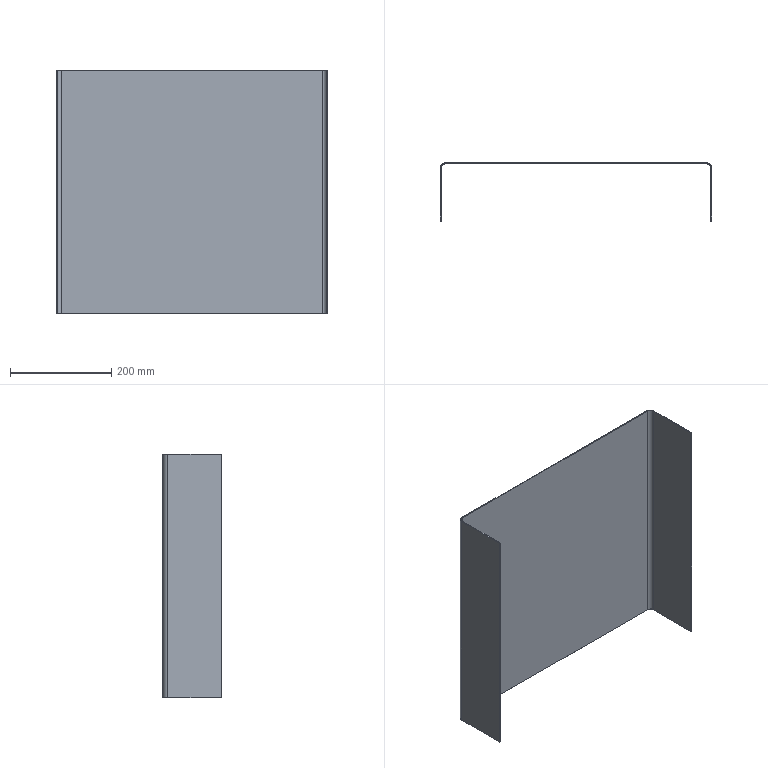Part | SolidWorks | features ExtruThin 1 | 1 solid | 14 faces | box 536 x 115.5 x 480 mm | volume 725063 mm3 | plane 10 | cylinder 4 | commonest cylinder face diameters 16 x2 20 x2
STEP:
#1=CARTESIAN_POINT('',(0.,-10.,0.));
#2=VERTEX_POINT('',#1);
#3=CARTESIAN_POINT('',(0.,-115.5,0.));
#4=VERTEX_POINT('',#3);
#5=CARTESIAN_POINT('',(0.,-10.,0.));
#6=DIRECTION('',(0.,-1.,0.));
#7=VECTOR('',#6,1000.);
#8=LINE('',#5,#7);
#9=EDGE_CURVE('',#2,#4,#8,.T.);
#10=ORIENTED_EDGE('',*,*,#9,.T.);
#11=CARTESIAN_POINT('',(0.,-115.5,480.));
#12=VERTEX_POINT('',#11);
#13=CARTESIAN_POINT('',(0.,-115.5,480.));
#14=DIRECTION('',(0.,0.,-1.));
#15=VECTOR('',#14,1000.);
#16=LINE('',#13,#15);
#17=EDGE_CURVE('',#12,#4,#16,.T.);
#18=ORIENTED_EDGE('',*,*,#17,.F.);
#19=CARTESIAN_POINT('',(0.,-10.,480.));
#20=VERTEX_POINT('',#19);
#21=CARTESIAN_POINT('',(0.,-10.,480.));
#22=DIRECTION('',(0.,-1.,0.));
#23=VECTOR('',#22,1000.);
#24=LINE('',#21,#23);
#25=EDGE_CURVE('',#20,#12,#24,.T.);
#26=ORIENTED_EDGE('',*,*,#25,.F.);
#27=CARTESIAN_POINT('',(0.,-10.,480.));
#28=DIRECTION('',(0.,0.,-1.));
#29=VECTOR('',#28,1000.);
#30=LINE('',#27,#29);
#31=EDGE_CURVE('',#20,#2,#30,.T.);
#32=ORIENTED_EDGE('',*,*,#31,.T.);
#33=EDGE_LOOP('',(#10,#18,#26,#32));
#34=FACE_OUTER_BOUND('',#33,.T.);
#35=CARTESIAN_POINT('',(0.,-10.,480.));
#36=DIRECTION('',(1.,0.,0.));
#37=DIRECTION('',(0.,1.,0.));
#38=AXIS2_PLACEMENT_3D('',#35,#36,#37);
#39=PLANE('',#38);
#40=ADVANCED_FACE('',(#34),#39,.F.);
#41=CARTESIAN_POINT('',(2.,-115.5,0.));
#42=VERTEX_POINT('',#41);
#43=CARTESIAN_POINT('',(2.,-115.5,0.));
#44=DIRECTION('',(-1.,0.,0.));
#45=VECTOR('',#44,1000.);
#46=LINE('',#43,#45);
#47=EDGE_CURVE('',#42,#4,#46,.T.);
#48=ORIENTED_EDGE('',*,*,#47,.F.);
#49=CARTESIAN_POINT('',(2.,-115.5,480.));
#50=VERTEX_POINT('',#49);
#51=CARTESIAN_POINT('',(2.,-115.5,480.));
#52=DIRECTION('',(0.,0.,-1.));
#53=VECTOR('',#52,1000.);
#54=LINE('',#51,#53);
#55=EDGE_CURVE('',#50,#42,#54,.T.);
#56=ORIENTED_EDGE('',*,*,#55,.F.);
#57=CARTESIAN_POINT('',(2.,-115.5,480.));
#58=DIRECTION('',(-1.,0.,0.));
#59=VECTOR('',#58,1000.);
#60=LINE('',#57,#59);
#61=EDGE_CURVE('',#50,#12,#60,.T.);
#62=ORIENTED_EDGE('',*,*,#61,.T.);
#63=ORIENTED_EDGE('',*,*,#17,.T.);
#64=EDGE_LOOP('',(#48,#56,#62,#63));
#65=FACE_OUTER_BOUND('',#64,.T.);
#66=CARTESIAN_POINT('',(2.,-115.5,480.));
#67=DIRECTION('',(0.,-1.,0.));
#68=DIRECTION('',(1.,0.,0.));
#69=AXIS2_PLACEMENT_3D('',#66,#67,#68);
#70=PLANE('',#69);
#71=ADVANCED_FACE('',(#65),#70,.T.);
#72=CARTESIAN_POINT('',(2.,-10.,0.));
#73=VERTEX_POINT('',#72);
#74=CARTESIAN_POINT('',(2.,-10.,0.));
#75=DIRECTION('',(0.,-1.,0.));
#76=VECTOR('',#75,1000.);
#77=LINE('',#74,#76);
#78=EDGE_CURVE('',#73,#42,#77,.T.);
#79=ORIENTED_EDGE('',*,*,#78,.F.);
#80=CARTESIAN_POINT('',(2.,-10.,480.));
#81=VERTEX_POINT('',#80);
#82=CARTESIAN_POINT('',(2.,-10.,480.));
#83=DIRECTION('',(0.,0.,-1.));
#84=VECTOR('',#83,1000.);
#85=LINE('',#82,#84);
#86=EDGE_CURVE('',#81,#73,#85,.T.);
#87=ORIENTED_EDGE('',*,*,#86,.F.);
#88=CARTESIAN_POINT('',(2.,-10.,480.));
#89=DIRECTION('',(0.,-1.,0.));
#90=VECTOR('',#89,1000.);
#91=LINE('',#88,#90);
#92=EDGE_CURVE('',#81,#50,#91,.T.);
#93=ORIENTED_EDGE('',*,*,#92,.T.);
#94=ORIENTED_EDGE('',*,*,#55,.T.);
#95=EDGE_LOOP('',(#79,#87,#93,#94));
#96=FACE_OUTER_BOUND('',#95,.T.);
#97=CARTESIAN_POINT('',(2.,-10.,480.));
#98=DIRECTION('',(1.,0.,0.));
#99=DIRECTION('',(0.,1.,0.));
#100=AXIS2_PLACEMENT_3D('',#97,#98,#99);
#101=PLANE('',#100);
#102=ADVANCED_FACE('',(#96),#101,.T.);
#103=CARTESIAN_POINT('',(10.,-2.,0.));
#104=VERTEX_POINT('',#103);
#105=CARTESIAN_POINT('',(10.,-10.,0.));
#106=DIRECTION('',(0.,0.,1.));
#107=DIRECTION('',(1.,0.,0.));
#108=AXIS2_PLACEMENT_3D('',#105,#106,#107);
#109=CIRCLE('',#108,8.);
#110=EDGE_CURVE('',#104,#73,#109,.T.);
#111=ORIENTED_EDGE('',*,*,#110,.F.);
#112=CARTESIAN_POINT('',(10.,-2.,480.));
#113=VERTEX_POINT('',#112);
#114=CARTESIAN_POINT('',(10.,-2.,480.));
#115=DIRECTION('',(0.,0.,-1.));
#116=VECTOR('',#115,1000.);
#117=LINE('',#114,#116);
#118=EDGE_CURVE('',#113,#104,#117,.T.);
#119=ORIENTED_EDGE('',*,*,#118,.F.);
#120=CARTESIAN_POINT('',(10.,-10.,480.));
#121=DIRECTION('',(0.,0.,1.));
#122=DIRECTION('',(1.,0.,0.));
#123=AXIS2_PLACEMENT_3D('',#120,#121,#122);
#124=CIRCLE('',#123,8.);
#125=EDGE_CURVE('',#113,#81,#124,.T.);
#126=ORIENTED_EDGE('',*,*,#125,.T.);
#127=ORIENTED_EDGE('',*,*,#86,.T.);
#128=EDGE_LOOP('',(#111,#119,#126,#127));
#129=FACE_OUTER_BOUND('',#128,.T.);
#130=CARTESIAN_POINT('',(10.,-10.,480.));
#131=DIRECTION('',(0.,0.,-1.));
#132=DIRECTION('',(-1.,0.,0.));
#133=AXIS2_PLACEMENT_3D('',#130,#131,#132);
#134=CYLINDRICAL_SURFACE('',#133,8.);
#135=ADVANCED_FACE('',(#129),#134,.F.);
#136=CARTESIAN_POINT('',(526.,-2.,0.));
#137=VERTEX_POINT('',#136);
#138=CARTESIAN_POINT('',(10.,-2.,0.));
#139=DIRECTION('',(-1.,0.,0.));
#140=VECTOR('',#139,1000.);
#141=LINE('',#138,#140);
#142=EDGE_CURVE('',#137,#104,#141,.T.);
#143=ORIENTED_EDGE('',*,*,#142,.F.);
#144=CARTESIAN_POINT('',(526.,-2.,480.));
#145=VERTEX_POINT('',#144);
#146=CARTESIAN_POINT('',(526.,-2.,480.));
#147=DIRECTION('',(0.,0.,-1.));
#148=VECTOR('',#147,1000.);
#149=LINE('',#146,#148);
#150=EDGE_CURVE('',#145,#137,#149,.T.);
#151=ORIENTED_EDGE('',*,*,#150,.F.);
#152=CARTESIAN_POINT('',(10.,-2.,480.));
#153=DIRECTION('',(-1.,0.,0.));
#154=VECTOR('',#153,1000.);
#155=LINE('',#152,#154);
#156=EDGE_CURVE('',#145,#113,#155,.T.);
#157=ORIENTED_EDGE('',*,*,#156,.T.);
#158=ORIENTED_EDGE('',*,*,#118,.T.);
#159=EDGE_LOOP('',(#143,#151,#157,#158));
#160=FACE_OUTER_BOUND('',#159,.T.);
#161=CARTESIAN_POINT('',(10.,-2.,480.));
#162=DIRECTION('',(0.,-1.,0.));
#163=DIRECTION('',(0.,0.,-1.));
#164=AXIS2_PLACEMENT_3D('',#161,#162,#163);
#165=PLANE('',#164);
#166=ADVANCED_FACE('',(#160),#165,.T.);
#167=CARTESIAN_POINT('',(534.,-10.,0.));
#168=VERTEX_POINT('',#167);
#169=CARTESIAN_POINT('',(526.,-10.,0.));
#170=DIRECTION('',(0.,0.,1.));
#171=DIRECTION('',(1.,0.,0.));
#172=AXIS2_PLACEMENT_3D('',#169,#170,#171);
#173=CIRCLE('',#172,8.);
#174=EDGE_CURVE('',#168,#137,#173,.T.);
#175=ORIENTED_EDGE('',*,*,#174,.F.);
#176=CARTESIAN_POINT('',(534.,-10.,480.));
#177=VERTEX_POINT('',#176);
#178=CARTESIAN_POINT('',(534.,-10.,480.));
#179=DIRECTION('',(0.,0.,-1.));
#180=VECTOR('',#179,1000.);
#181=LINE('',#178,#180);
#182=EDGE_CURVE('',#177,#168,#181,.T.);
#183=ORIENTED_EDGE('',*,*,#182,.F.);
#184=CARTESIAN_POINT('',(526.,-10.,480.));
#185=DIRECTION('',(0.,0.,1.));
#186=DIRECTION('',(1.,0.,0.));
#187=AXIS2_PLACEMENT_3D('',#184,#185,#186);
#188=CIRCLE('',#187,8.);
#189=EDGE_CURVE('',#177,#145,#188,.T.);
#190=ORIENTED_EDGE('',*,*,#189,.T.);
#191=ORIENTED_EDGE('',*,*,#150,.T.);
#192=EDGE_LOOP('',(#175,#183,#190,#191));
#193=FACE_OUTER_BOUND('',#192,.T.);
#194=CARTESIAN_POINT('',(526.,-10.,480.));
#195=DIRECTION('',(0.,0.,-1.));
#196=DIRECTION('',(-1.,0.,0.));
#197=AXIS2_PLACEMENT_3D('',#194,#195,#196);
#198=CYLINDRICAL_SURFACE('',#197,8.);
#199=ADVANCED_FACE('',(#193),#198,.F.);
#200=CARTESIAN_POINT('',(534.,-115.5,0.));
#201=VERTEX_POINT('',#200);
#202=CARTESIAN_POINT('',(534.,-10.,0.));
#203=DIRECTION('',(0.,1.,0.));
#204=VECTOR('',#203,1000.);
#205=LINE('',#202,#204);
#206=EDGE_CURVE('',#201,#168,#205,.T.);
#207=ORIENTED_EDGE('',*,*,#206,.F.);
#208=CARTESIAN_POINT('',(534.,-115.5,480.));
#209=VERTEX_POINT('',#208);
#210=CARTESIAN_POINT('',(534.,-115.5,480.));
#211=DIRECTION('',(0.,0.,-1.));
#212=VECTOR('',#211,1000.);
#213=LINE('',#210,#212);
#214=EDGE_CURVE('',#209,#201,#213,.T.);
#215=ORIENTED_EDGE('',*,*,#214,.F.);
#216=CARTESIAN_POINT('',(534.,-10.,480.));
#217=DIRECTION('',(0.,1.,0.));
#218=VECTOR('',#217,1000.);
#219=LINE('',#216,#218);
#220=EDGE_CURVE('',#209,#177,#219,.T.);
#221=ORIENTED_EDGE('',*,*,#220,.T.);
#222=ORIENTED_EDGE('',*,*,#182,.T.);
#223=EDGE_LOOP('',(#207,#215,#221,#222));
#224=FACE_OUTER_BOUND('',#223,.T.);
#225=CARTESIAN_POINT('',(534.,-10.,480.));
#226=DIRECTION('',(-1.,0.,0.));
#227=DIRECTION('',(0.,0.,1.));
#228=AXIS2_PLACEMENT_3D('',#225,#226,#227);
#229=PLANE('',#228);
#230=ADVANCED_FACE('',(#224),#229,.T.);
#231=CARTESIAN_POINT('',(536.,-115.5,0.));
#232=VERTEX_POINT('',#231);
#233=CARTESIAN_POINT('',(536.,-115.5,0.));
#234=DIRECTION('',(-1.,0.,0.));
#235=VECTOR('',#234,1000.);
#236=LINE('',#233,#235);
#237=EDGE_CURVE('',#232,#201,#236,.T.);
#238=ORIENTED_EDGE('',*,*,#237,.F.);
#239=CARTESIAN_POINT('',(536.,-115.5,480.));
#240=VERTEX_POINT('',#239);
#241=CARTESIAN_POINT('',(536.,-115.5,480.));
#242=DIRECTION('',(0.,0.,-1.));
#243=VECTOR('',#242,1000.);
#244=LINE('',#241,#243);
#245=EDGE_CURVE('',#240,#232,#244,.T.);
#246=ORIENTED_EDGE('',*,*,#245,.F.);
#247=CARTESIAN_POINT('',(536.,-115.5,480.));
#248=DIRECTION('',(-1.,0.,0.));
#249=VECTOR('',#248,1000.);
#250=LINE('',#247,#249);
#251=EDGE_CURVE('',#240,#209,#250,.T.);
#252=ORIENTED_EDGE('',*,*,#251,.T.);
#253=ORIENTED_EDGE('',*,*,#214,.T.);
#254=EDGE_LOOP('',(#238,#246,#252,#253));
#255=FACE_OUTER_BOUND('',#254,.T.);
#256=CARTESIAN_POINT('',(536.,-115.5,480.));
#257=DIRECTION('',(0.,-1.,0.));
#258=DIRECTION('',(0.,0.,-1.));
#259=AXIS2_PLACEMENT_3D('',#256,#257,#258);
#260=PLANE('',#259);
#261=ADVANCED_FACE('',(#255),#260,.T.);
#262=CARTESIAN_POINT('',(536.,-10.,0.));
#263=VERTEX_POINT('',#262);
#264=CARTESIAN_POINT('',(536.,-10.,0.));
#265=DIRECTION('',(0.,1.,0.));
#266=VECTOR('',#265,1000.);
#267=LINE('',#264,#266);
#268=EDGE_CURVE('',#232,#263,#267,.T.);
#269=ORIENTED_EDGE('',*,*,#268,.T.);
#270=CARTESIAN_POINT('',(536.,-10.,480.));
#271=VERTEX_POINT('',#270);
#272=CARTESIAN_POINT('',(536.,-10.,480.));
#273=DIRECTION('',(0.,0.,-1.));
#274=VECTOR('',#273,1000.);
#275=LINE('',#272,#274);
#276=EDGE_CURVE('',#271,#263,#275,.T.);
#277=ORIENTED_EDGE('',*,*,#276,.F.);
#278=CARTESIAN_POINT('',(536.,-10.,480.));
#279=DIRECTION('',(0.,1.,0.));
#280=VECTOR('',#279,1000.);
#281=LINE('',#278,#280);
#282=EDGE_CURVE('',#240,#271,#281,.T.);
#283=ORIENTED_EDGE('',*,*,#282,.F.);
#284=ORIENTED_EDGE('',*,*,#245,.T.);
#285=EDGE_LOOP('',(#269,#277,#283,#284));
#286=FACE_OUTER_BOUND('',#285,.T.);
#287=CARTESIAN_POINT('',(536.,-10.,480.));
#288=DIRECTION('',(-1.,0.,0.));
#289=DIRECTION('',(0.,0.,1.));
#290=AXIS2_PLACEMENT_3D('',#287,#288,#289);
#291=PLANE('',#290);
#292=ADVANCED_FACE('',(#286),#291,.F.);
#293=CARTESIAN_POINT('',(526.,0.,0.));
#294=VERTEX_POINT('',#293);
#295=CARTESIAN_POINT('',(526.,-10.,0.));
#296=DIRECTION('',(0.,0.,1.));
#297=DIRECTION('',(1.,0.,0.));
#298=AXIS2_PLACEMENT_3D('',#295,#296,#297);
#299=CIRCLE('',#298,10.);
#300=EDGE_CURVE('',#263,#294,#299,.T.);
#301=ORIENTED_EDGE('',*,*,#300,.T.);
#302=CARTESIAN_POINT('',(526.,0.,480.));
#303=VERTEX_POINT('',#302);
#304=CARTESIAN_POINT('',(526.,0.,480.));
#305=DIRECTION('',(0.,0.,-1.));
#306=VECTOR('',#305,1000.);
#307=LINE('',#304,#306);
#308=EDGE_CURVE('',#303,#294,#307,.T.);
#309=ORIENTED_EDGE('',*,*,#308,.F.);
#310=CARTESIAN_POINT('',(526.,-10.,480.));
#311=DIRECTION('',(0.,0.,1.));
#312=DIRECTION('',(1.,0.,0.));
#313=AXIS2_PLACEMENT_3D('',#310,#311,#312);
#314=CIRCLE('',#313,10.);
#315=EDGE_CURVE('',#271,#303,#314,.T.);
#316=ORIENTED_EDGE('',*,*,#315,.F.);
#317=ORIENTED_EDGE('',*,*,#276,.T.);
#318=EDGE_LOOP('',(#301,#309,#316,#317));
#319=FACE_OUTER_BOUND('',#318,.T.);
#320=CARTESIAN_POINT('',(526.,-10.,480.));
#321=DIRECTION('',(0.,0.,-1.));
#322=DIRECTION('',(-1.,0.,0.));
#323=AXIS2_PLACEMENT_3D('',#320,#321,#322);
#324=CYLINDRICAL_SURFACE('',#323,10.);
#325=ADVANCED_FACE('',(#319),#324,.T.);
#326=CARTESIAN_POINT('',(10.,0.,0.));
#327=VERTEX_POINT('',#326);
#328=CARTESIAN_POINT('',(10.,0.,0.));
#329=DIRECTION('',(-1.,0.,0.));
#330=VECTOR('',#329,1000.);
#331=LINE('',#328,#330);
#332=EDGE_CURVE('',#294,#327,#331,.T.);
#333=ORIENTED_EDGE('',*,*,#332,.T.);
#334=CARTESIAN_POINT('',(10.,0.,480.));
#335=VERTEX_POINT('',#334);
#336=CARTESIAN_POINT('',(10.,0.,480.));
#337=DIRECTION('',(0.,0.,-1.));
#338=VECTOR('',#337,1000.);
#339=LINE('',#336,#338);
#340=EDGE_CURVE('',#335,#327,#339,.T.);
#341=ORIENTED_EDGE('',*,*,#340,.F.);
#342=CARTESIAN_POINT('',(10.,0.,480.));
#343=DIRECTION('',(-1.,0.,0.));
#344=VECTOR('',#343,1000.);
#345=LINE('',#342,#344);
#346=EDGE_CURVE('',#303,#335,#345,.T.);
#347=ORIENTED_EDGE('',*,*,#346,.F.);
#348=ORIENTED_EDGE('',*,*,#308,.T.);
#349=EDGE_LOOP('',(#333,#341,#347,#348));
#350=FACE_OUTER_BOUND('',#349,.T.);
#351=CARTESIAN_POINT('',(10.,0.,480.));
#352=DIRECTION('',(0.,-1.,0.));
#353=DIRECTION('',(0.,0.,-1.));
#354=AXIS2_PLACEMENT_3D('',#351,#352,#353);
#355=PLANE('',#354);
#356=ADVANCED_FACE('',(#350),#355,.F.);
#357=CARTESIAN_POINT('',(10.,-10.,0.));
#358=DIRECTION('',(0.,0.,1.));
#359=DIRECTION('',(1.,0.,0.));
#360=AXIS2_PLACEMENT_3D('',#357,#358,#359);
#361=CIRCLE('',#360,10.);
#362=EDGE_CURVE('',#327,#2,#361,.T.);
#363=ORIENTED_EDGE('',*,*,#362,.T.);
#364=ORIENTED_EDGE('',*,*,#31,.F.);
#365=CARTESIAN_POINT('',(10.,-10.,480.));
#366=DIRECTION('',(0.,0.,1.));
#367=DIRECTION('',(1.,0.,0.));
#368=AXIS2_PLACEMENT_3D('',#365,#366,#367);
#369=CIRCLE('',#368,10.);
#370=EDGE_CURVE('',#335,#20,#369,.T.);
#371=ORIENTED_EDGE('',*,*,#370,.F.);
#372=ORIENTED_EDGE('',*,*,#340,.T.);
#373=EDGE_LOOP('',(#363,#364,#371,#372));
#374=FACE_OUTER_BOUND('',#373,.T.);
#375=CARTESIAN_POINT('',(10.,-10.,480.));
#376=DIRECTION('',(0.,0.,-1.));
#377=DIRECTION('',(-1.,0.,0.));
#378=AXIS2_PLACEMENT_3D('',#375,#376,#377);
#379=CYLINDRICAL_SURFACE('',#378,10.);
#380=ADVANCED_FACE('',(#374),#379,.T.);
#381=ORIENTED_EDGE('',*,*,#25,.T.);
#382=ORIENTED_EDGE('',*,*,#61,.F.);
#383=ORIENTED_EDGE('',*,*,#92,.F.);
#384=ORIENTED_EDGE('',*,*,#125,.F.);
#385=ORIENTED_EDGE('',*,*,#156,.F.);
#386=ORIENTED_EDGE('',*,*,#189,.F.);
#387=ORIENTED_EDGE('',*,*,#220,.F.);
#388=ORIENTED_EDGE('',*,*,#251,.F.);
#389=ORIENTED_EDGE('',*,*,#282,.T.);
#390=ORIENTED_EDGE('',*,*,#315,.T.);
#391=ORIENTED_EDGE('',*,*,#346,.T.);
#392=ORIENTED_EDGE('',*,*,#370,.T.);
#393=EDGE_LOOP('',(#381,#382,#383,#384,#385,#386,#387,#388,#389,#390,#391,#392));
#394=FACE_OUTER_BOUND('',#393,.T.);
#395=CARTESIAN_POINT('',(10.,-10.,480.));
#396=DIRECTION('',(0.,0.,1.));
#397=DIRECTION('',(1.,0.,0.));
#398=AXIS2_PLACEMENT_3D('',#395,#396,#397);
#399=PLANE('',#398);
#400=ADVANCED_FACE('',(#394),#399,.T.);
#401=ORIENTED_EDGE('',*,*,#9,.F.);
#402=ORIENTED_EDGE('',*,*,#362,.F.);
#403=ORIENTED_EDGE('',*,*,#332,.F.);
#404=ORIENTED_EDGE('',*,*,#300,.F.);
#405=ORIENTED_EDGE('',*,*,#268,.F.);
#406=ORIENTED_EDGE('',*,*,#237,.T.);
#407=ORIENTED_EDGE('',*,*,#206,.T.);
#408=ORIENTED_EDGE('',*,*,#174,.T.);
#409=ORIENTED_EDGE('',*,*,#142,.T.);
#410=ORIENTED_EDGE('',*,*,#110,.T.);
#411=ORIENTED_EDGE('',*,*,#78,.T.);
#412=ORIENTED_EDGE('',*,*,#47,.T.);
#413=EDGE_LOOP('',(#401,#402,#403,#404,#405,#406,#407,#408,#409,#410,#411,#412));
#414=FACE_OUTER_BOUND('',#413,.T.);
#415=CARTESIAN_POINT('',(10.,-10.,0.));
#416=DIRECTION('',(0.,0.,1.));
#417=DIRECTION('',(1.,0.,0.));
#418=AXIS2_PLACEMENT_3D('',#415,#416,#417);
#419=PLANE('',#418);
#420=ADVANCED_FACE('',(#414),#419,.F.);
#421=CLOSED_SHELL('',(#40,#71,#102,#135,#166,#199,#230,#261,#292,#325,#356,#380,#400,#420));
#422=MANIFOLD_SOLID_BREP('',#421);
#423=CARTESIAN_POINT('',(0.,0.,0.));
#424=DIRECTION('',(0.,0.,1.));
#425=DIRECTION('',(1.,0.,0.));
#426=AXIS2_PLACEMENT_3D('',#423,#424,#425);
#427=(LENGTH_UNIT()NAMED_UNIT(*)SI_UNIT(.MILLI.,.METRE.));
#428=UNCERTAINTY_MEASURE_WITH_UNIT(LENGTH_MEASURE(0.00001),#427,'','');
#429=(NAMED_UNIT(*)PLANE_ANGLE_UNIT()SI_UNIT($,.RADIAN.));
#430=(NAMED_UNIT(*)SI_UNIT($,.STERADIAN.)SOLID_ANGLE_UNIT());
#431=(GEOMETRIC_REPRESENTATION_CONTEXT(3)GLOBAL_UNCERTAINTY_ASSIGNED_CONTEXT((#428))GLOBAL_UNIT_ASSIGNED_CONTEXT((#427,#429,#430))REPRESENTATION_CONTEXT('',''));
#432=ADVANCED_BREP_SHAPE_REPRESENTATION('',(#422,#426),#431);